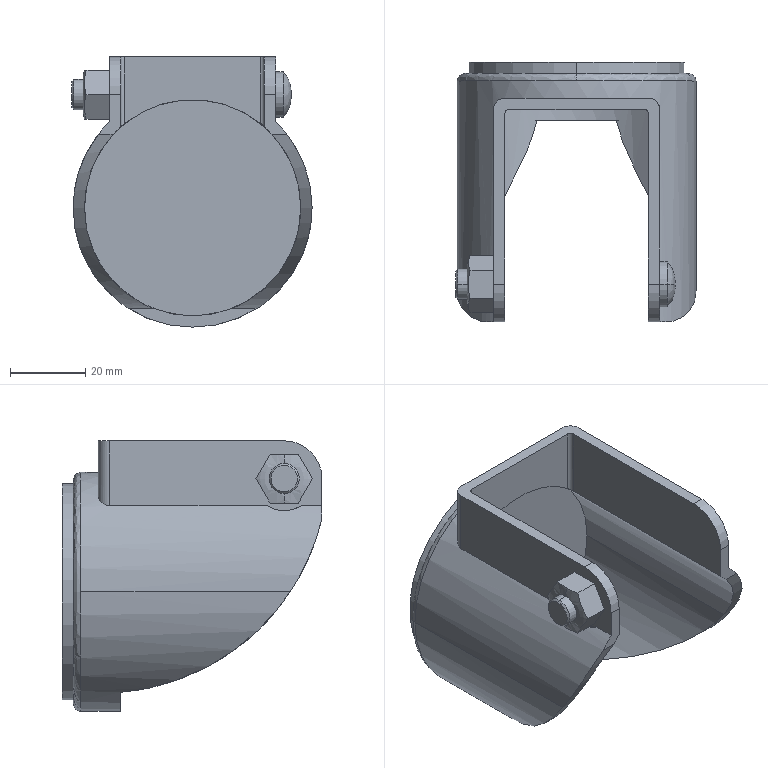Part | STEP file | 1 solid | 48 faces | box 63.667 x 68.9 x 71.667 mm | volume 52181 mm3 | cylinder 20 | plane 20 | spline 6 | cone 2 | commonest cylinder face diameters 57.333 x4 2 x2 6 x2 8 x2 12 x2 17 x2